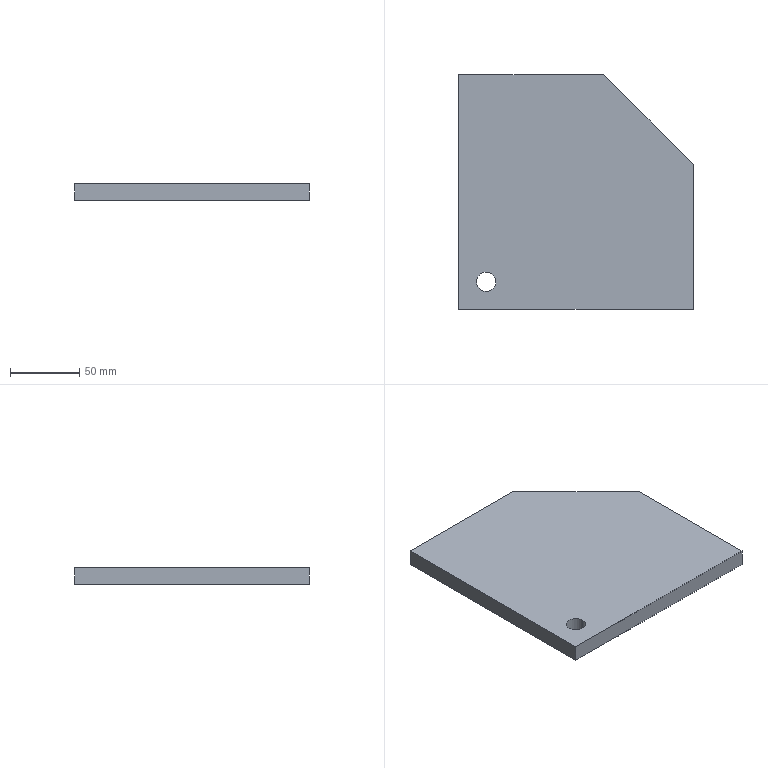Part | SolidWorks | features HoleWzd 2, Chamfer 1, Extrusion 1 | 1 solid | 9 faces | box 170 x 170 x 12 mm | volume 319603 mm3 | plane 7 | cylinder 2 | commonest cylinder face diameters 14 x2
STEP:
#1=CARTESIAN_POINT('',(13.,20.,-12.));
#2=VERTEX_POINT('',#1);
#3=CARTESIAN_POINT('',(27.,20.,-12.));
#4=VERTEX_POINT('',#3);
#5=CARTESIAN_POINT('',(20.,20.,-12.));
#6=DIRECTION('',(0.,0.,1.));
#7=DIRECTION('',(1.,0.,0.));
#8=AXIS2_PLACEMENT_3D('',#5,#6,#7);
#9=CIRCLE('',#8,7.);
#10=EDGE_CURVE('',#2,#4,#9,.T.);
#11=ORIENTED_EDGE('',*,*,#10,.F.);
#12=CARTESIAN_POINT('',(13.,20.,0.));
#13=VERTEX_POINT('',#12);
#14=CARTESIAN_POINT('',(13.,20.,0.));
#15=DIRECTION('',(0.,0.,1.));
#16=VECTOR('',#15,1000.);
#17=LINE('',#14,#16);
#18=EDGE_CURVE('',#2,#13,#17,.T.);
#19=ORIENTED_EDGE('',*,*,#18,.T.);
#20=CARTESIAN_POINT('',(27.,20.,0.));
#21=VERTEX_POINT('',#20);
#22=CARTESIAN_POINT('',(20.,20.,0.));
#23=DIRECTION('',(0.,0.,1.));
#24=DIRECTION('',(1.,0.,0.));
#25=AXIS2_PLACEMENT_3D('',#22,#23,#24);
#26=CIRCLE('',#25,7.);
#27=EDGE_CURVE('',#13,#21,#26,.T.);
#28=ORIENTED_EDGE('',*,*,#27,.T.);
#29=CARTESIAN_POINT('',(27.,20.,0.));
#30=DIRECTION('',(0.,0.,1.));
#31=VECTOR('',#30,1000.);
#32=LINE('',#29,#31);
#33=EDGE_CURVE('',#4,#21,#32,.T.);
#34=ORIENTED_EDGE('',*,*,#33,.F.);
#35=EDGE_LOOP('',(#11,#19,#28,#34));
#36=FACE_OUTER_BOUND('',#35,.T.);
#37=CARTESIAN_POINT('',(20.,20.,0.));
#38=DIRECTION('',(0.,0.,1.));
#39=DIRECTION('',(1.,0.,0.));
#40=AXIS2_PLACEMENT_3D('',#37,#38,#39);
#41=CYLINDRICAL_SURFACE('',#40,7.);
#42=ADVANCED_FACE('',(#36),#41,.F.);
#43=CARTESIAN_POINT('',(170.,0.,-12.));
#44=VERTEX_POINT('',#43);
#45=CARTESIAN_POINT('',(170.,105.,-12.));
#46=VERTEX_POINT('',#45);
#47=CARTESIAN_POINT('',(170.,0.,-12.));
#48=DIRECTION('',(0.,1.,0.));
#49=VECTOR('',#48,1000.);
#50=LINE('',#47,#49);
#51=EDGE_CURVE('',#44,#46,#50,.T.);
#52=ORIENTED_EDGE('',*,*,#51,.T.);
#53=CARTESIAN_POINT('',(170.,105.,0.));
#54=VERTEX_POINT('',#53);
#55=CARTESIAN_POINT('',(170.,105.,-12.));
#56=DIRECTION('',(0.,0.,1.));
#57=VECTOR('',#56,1000.);
#58=LINE('',#55,#57);
#59=EDGE_CURVE('',#46,#54,#58,.T.);
#60=ORIENTED_EDGE('',*,*,#59,.T.);
#61=CARTESIAN_POINT('',(170.,0.,0.));
#62=VERTEX_POINT('',#61);
#63=CARTESIAN_POINT('',(170.,0.,0.));
#64=DIRECTION('',(0.,1.,0.));
#65=VECTOR('',#64,1000.);
#66=LINE('',#63,#65);
#67=EDGE_CURVE('',#62,#54,#66,.T.);
#68=ORIENTED_EDGE('',*,*,#67,.F.);
#69=CARTESIAN_POINT('',(170.,0.,-12.));
#70=DIRECTION('',(0.,0.,1.));
#71=VECTOR('',#70,1000.);
#72=LINE('',#69,#71);
#73=EDGE_CURVE('',#44,#62,#72,.T.);
#74=ORIENTED_EDGE('',*,*,#73,.F.);
#75=EDGE_LOOP('',(#52,#60,#68,#74));
#76=FACE_OUTER_BOUND('',#75,.T.);
#77=CARTESIAN_POINT('',(170.,0.,-12.));
#78=DIRECTION('',(1.,0.,0.));
#79=DIRECTION('',(0.,0.,-1.));
#80=AXIS2_PLACEMENT_3D('',#77,#78,#79);
#81=PLANE('',#80);
#82=ADVANCED_FACE('',(#76),#81,.T.);
#83=CARTESIAN_POINT('',(0.,0.,0.));
#84=VERTEX_POINT('',#83);
#85=CARTESIAN_POINT('',(0.,0.,0.));
#86=DIRECTION('',(1.,0.,0.));
#87=VECTOR('',#86,1000.);
#88=LINE('',#85,#87);
#89=EDGE_CURVE('',#84,#62,#88,.T.);
#90=ORIENTED_EDGE('',*,*,#89,.F.);
#91=CARTESIAN_POINT('',(0.,0.,-12.));
#92=VERTEX_POINT('',#91);
#93=CARTESIAN_POINT('',(0.,0.,-12.));
#94=DIRECTION('',(0.,0.,1.));
#95=VECTOR('',#94,1000.);
#96=LINE('',#93,#95);
#97=EDGE_CURVE('',#92,#84,#96,.T.);
#98=ORIENTED_EDGE('',*,*,#97,.F.);
#99=CARTESIAN_POINT('',(0.,0.,-12.));
#100=DIRECTION('',(1.,0.,0.));
#101=VECTOR('',#100,1000.);
#102=LINE('',#99,#101);
#103=EDGE_CURVE('',#92,#44,#102,.T.);
#104=ORIENTED_EDGE('',*,*,#103,.T.);
#105=ORIENTED_EDGE('',*,*,#73,.T.);
#106=EDGE_LOOP('',(#90,#98,#104,#105));
#107=FACE_OUTER_BOUND('',#106,.T.);
#108=CARTESIAN_POINT('',(0.,0.,-12.));
#109=DIRECTION('',(0.,-1.,0.));
#110=DIRECTION('',(0.,0.,-1.));
#111=AXIS2_PLACEMENT_3D('',#108,#109,#110);
#112=PLANE('',#111);
#113=ADVANCED_FACE('',(#107),#112,.T.);
#114=CARTESIAN_POINT('',(0.,170.,0.));
#115=VERTEX_POINT('',#114);
#116=CARTESIAN_POINT('',(0.,0.,0.));
#117=DIRECTION('',(0.,-1.,0.));
#118=VECTOR('',#117,1000.);
#119=LINE('',#116,#118);
#120=EDGE_CURVE('',#115,#84,#119,.T.);
#121=ORIENTED_EDGE('',*,*,#120,.F.);
#122=CARTESIAN_POINT('',(0.,170.,-12.));
#123=VERTEX_POINT('',#122);
#124=CARTESIAN_POINT('',(0.,170.,-12.));
#125=DIRECTION('',(0.,0.,1.));
#126=VECTOR('',#125,1000.);
#127=LINE('',#124,#126);
#128=EDGE_CURVE('',#123,#115,#127,.T.);
#129=ORIENTED_EDGE('',*,*,#128,.F.);
#130=CARTESIAN_POINT('',(0.,0.,-12.));
#131=DIRECTION('',(0.,-1.,0.));
#132=VECTOR('',#131,1000.);
#133=LINE('',#130,#132);
#134=EDGE_CURVE('',#123,#92,#133,.T.);
#135=ORIENTED_EDGE('',*,*,#134,.T.);
#136=ORIENTED_EDGE('',*,*,#97,.T.);
#137=EDGE_LOOP('',(#121,#129,#135,#136));
#138=FACE_OUTER_BOUND('',#137,.T.);
#139=CARTESIAN_POINT('',(0.,0.,-12.));
#140=DIRECTION('',(-1.,0.,0.));
#141=DIRECTION('',(0.,0.,1.));
#142=AXIS2_PLACEMENT_3D('',#139,#140,#141);
#143=PLANE('',#142);
#144=ADVANCED_FACE('',(#138),#143,.T.);
#145=CARTESIAN_POINT('',(105.,170.,0.));
#146=VERTEX_POINT('',#145);
#147=CARTESIAN_POINT('',(0.,170.,0.));
#148=DIRECTION('',(-1.,0.,0.));
#149=VECTOR('',#148,1000.);
#150=LINE('',#147,#149);
#151=EDGE_CURVE('',#146,#115,#150,.T.);
#152=ORIENTED_EDGE('',*,*,#151,.F.);
#153=CARTESIAN_POINT('',(105.,170.,-12.));
#154=VERTEX_POINT('',#153);
#155=CARTESIAN_POINT('',(105.,170.,-12.));
#156=DIRECTION('',(0.,0.,-1.));
#157=VECTOR('',#156,1000.);
#158=LINE('',#155,#157);
#159=EDGE_CURVE('',#146,#154,#158,.T.);
#160=ORIENTED_EDGE('',*,*,#159,.T.);
#161=CARTESIAN_POINT('',(0.,170.,-12.));
#162=DIRECTION('',(-1.,0.,0.));
#163=VECTOR('',#162,1000.);
#164=LINE('',#161,#163);
#165=EDGE_CURVE('',#154,#123,#164,.T.);
#166=ORIENTED_EDGE('',*,*,#165,.T.);
#167=ORIENTED_EDGE('',*,*,#128,.T.);
#168=EDGE_LOOP('',(#152,#160,#166,#167));
#169=FACE_OUTER_BOUND('',#168,.T.);
#170=CARTESIAN_POINT('',(0.,170.,-12.));
#171=DIRECTION('',(0.,1.,0.));
#172=DIRECTION('',(0.,0.,1.));
#173=AXIS2_PLACEMENT_3D('',#170,#171,#172);
#174=PLANE('',#173);
#175=ADVANCED_FACE('',(#169),#174,.T.);
#176=CARTESIAN_POINT('',(20.,20.,-12.));
#177=DIRECTION('',(0.,0.,1.));
#178=DIRECTION('',(1.,0.,0.));
#179=AXIS2_PLACEMENT_3D('',#176,#177,#178);
#180=CIRCLE('',#179,7.);
#181=EDGE_CURVE('',#4,#2,#180,.T.);
#182=ORIENTED_EDGE('',*,*,#181,.T.);
#183=ORIENTED_EDGE('',*,*,#10,.T.);
#184=EDGE_LOOP('',(#182,#183));
#185=FACE_BOUND('',#184,.T.);
#186=ORIENTED_EDGE('',*,*,#165,.F.);
#187=CARTESIAN_POINT('',(137.5,137.5,-12.));
#188=DIRECTION('',(0.7071,-0.7071,0.));
#189=VECTOR('',#188,1000.);
#190=LINE('',#187,#189);
#191=EDGE_CURVE('',#154,#46,#190,.T.);
#192=ORIENTED_EDGE('',*,*,#191,.T.);
#193=ORIENTED_EDGE('',*,*,#51,.F.);
#194=ORIENTED_EDGE('',*,*,#103,.F.);
#195=ORIENTED_EDGE('',*,*,#134,.F.);
#196=EDGE_LOOP('',(#186,#192,#193,#194,#195));
#197=FACE_OUTER_BOUND('',#196,.T.);
#198=CARTESIAN_POINT('',(170.,170.,-12.));
#199=DIRECTION('',(0.,0.,-1.));
#200=DIRECTION('',(-1.,0.,0.));
#201=AXIS2_PLACEMENT_3D('',#198,#199,#200);
#202=PLANE('',#201);
#203=ADVANCED_FACE('',(#185,#197),#202,.T.);
#204=CARTESIAN_POINT('',(20.,20.,0.));
#205=DIRECTION('',(0.,0.,1.));
#206=DIRECTION('',(1.,0.,0.));
#207=AXIS2_PLACEMENT_3D('',#204,#205,#206);
#208=CIRCLE('',#207,7.);
#209=EDGE_CURVE('',#21,#13,#208,.T.);
#210=ORIENTED_EDGE('',*,*,#209,.F.);
#211=ORIENTED_EDGE('',*,*,#27,.F.);
#212=EDGE_LOOP('',(#210,#211));
#213=FACE_BOUND('',#212,.T.);
#214=ORIENTED_EDGE('',*,*,#67,.T.);
#215=CARTESIAN_POINT('',(170.,105.,0.));
#216=DIRECTION('',(-0.7071,0.7071,0.));
#217=VECTOR('',#216,1000.);
#218=LINE('',#215,#217);
#219=EDGE_CURVE('',#54,#146,#218,.T.);
#220=ORIENTED_EDGE('',*,*,#219,.T.);
#221=ORIENTED_EDGE('',*,*,#151,.T.);
#222=ORIENTED_EDGE('',*,*,#120,.T.);
#223=ORIENTED_EDGE('',*,*,#89,.T.);
#224=EDGE_LOOP('',(#214,#220,#221,#222,#223));
#225=FACE_OUTER_BOUND('',#224,.T.);
#226=CARTESIAN_POINT('',(170.,170.,0.));
#227=DIRECTION('',(0.,0.,-1.));
#228=DIRECTION('',(-1.,0.,0.));
#229=AXIS2_PLACEMENT_3D('',#226,#227,#228);
#230=PLANE('',#229);
#231=ADVANCED_FACE('',(#213,#225),#230,.F.);
#232=ORIENTED_EDGE('',*,*,#18,.F.);
#233=ORIENTED_EDGE('',*,*,#181,.F.);
#234=ORIENTED_EDGE('',*,*,#33,.T.);
#235=ORIENTED_EDGE('',*,*,#209,.T.);
#236=EDGE_LOOP('',(#232,#233,#234,#235));
#237=FACE_OUTER_BOUND('',#236,.T.);
#238=CARTESIAN_POINT('',(20.,20.,0.));
#239=DIRECTION('',(0.,0.,1.));
#240=DIRECTION('',(1.,0.,0.));
#241=AXIS2_PLACEMENT_3D('',#238,#239,#240);
#242=CYLINDRICAL_SURFACE('',#241,7.);
#243=ADVANCED_FACE('',(#237),#242,.F.);
#244=ORIENTED_EDGE('',*,*,#191,.F.);
#245=ORIENTED_EDGE('',*,*,#159,.F.);
#246=ORIENTED_EDGE('',*,*,#219,.F.);
#247=ORIENTED_EDGE('',*,*,#59,.F.);
#248=EDGE_LOOP('',(#244,#245,#246,#247));
#249=FACE_OUTER_BOUND('',#248,.T.);
#250=CARTESIAN_POINT('',(170.,105.,-12.));
#251=DIRECTION('',(-0.7071,-0.7071,0.));
#252=DIRECTION('',(0.7071,-0.7071,0.));
#253=AXIS2_PLACEMENT_3D('',#250,#251,#252);
#254=PLANE('',#253);
#255=ADVANCED_FACE('',(#249),#254,.F.);
#256=CLOSED_SHELL('',(#42,#82,#113,#144,#175,#203,#231,#243,#255));
#257=MANIFOLD_SOLID_BREP('',#256);
#258=CARTESIAN_POINT('',(0.,0.,0.));
#259=DIRECTION('',(0.,0.,1.));
#260=DIRECTION('',(1.,0.,0.));
#261=AXIS2_PLACEMENT_3D('',#258,#259,#260);
#262=(LENGTH_UNIT()NAMED_UNIT(*)SI_UNIT(.MILLI.,.METRE.));
#263=UNCERTAINTY_MEASURE_WITH_UNIT(LENGTH_MEASURE(0.00001),#262,'','');
#264=(NAMED_UNIT(*)PLANE_ANGLE_UNIT()SI_UNIT($,.RADIAN.));
#265=(NAMED_UNIT(*)SI_UNIT($,.STERADIAN.)SOLID_ANGLE_UNIT());
#266=(GEOMETRIC_REPRESENTATION_CONTEXT(3)GLOBAL_UNCERTAINTY_ASSIGNED_CONTEXT((#263))GLOBAL_UNIT_ASSIGNED_CONTEXT((#262,#264,#265))REPRESENTATION_CONTEXT('',''));
#267=ADVANCED_BREP_SHAPE_REPRESENTATION('',(#257,#261),#266);